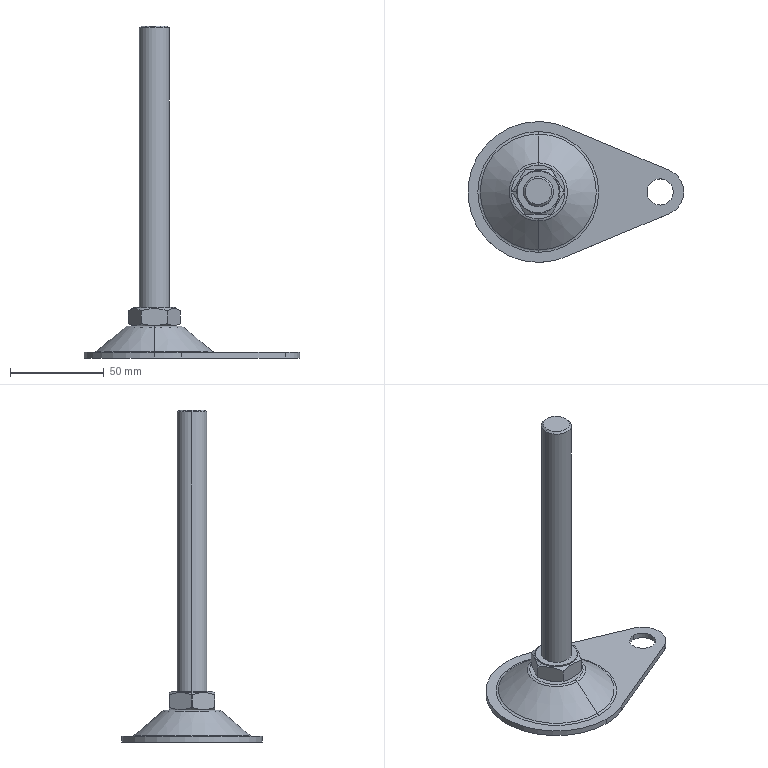Part | STEP file | ~PA16-150_1.stp | 1 solid | 51 faces | box 115 x 75 x 177 mm | volume 55978 mm3 | cylinder 19 | plane 16 | cone 10 | torus 6 | commonest cylinder face diameters 27.7 x7 75 x3 14 x2 16 x2 18 x2 22.3 x2